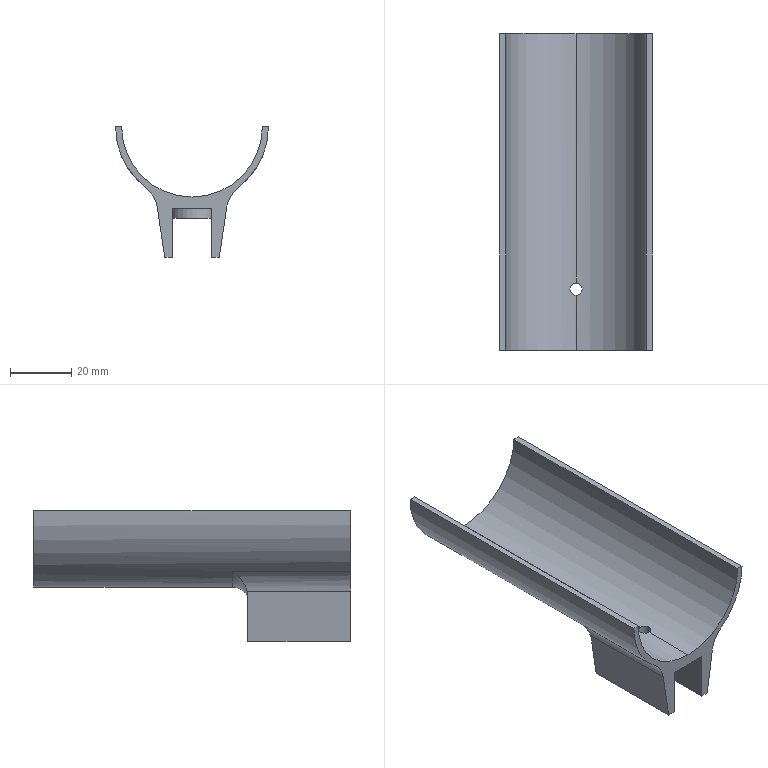Part | STEP file | Weighing slot | 1 solid | 27 faces | box 50 x 103.5 x 42.709 mm | volume 22376 mm3 | plane 15 | cylinder 10 | torus 2 | commonest cylinder face diameters 4 x2 14.095 x2 20 x2 46 x2 50 x2